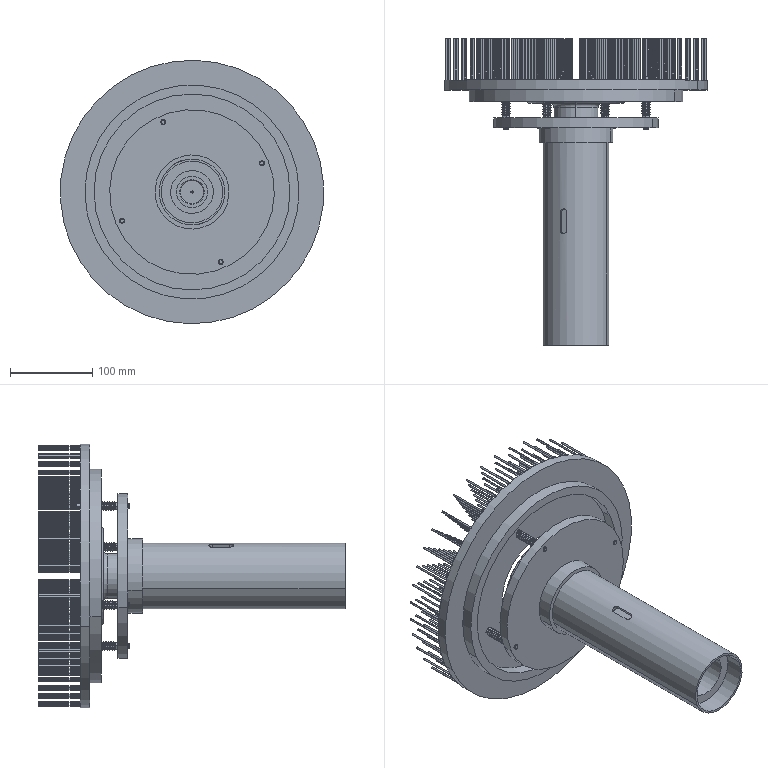Part | NX | features BREP 11 | 23 solids | 1564 faces | box 320 x 372 x 320 mm | volume 2233372 mm3 | cylinder 1010 | plane 502 | cone 32 | torus 12 | spline 8 | commonest cylinder face diameters 2 x800 2.5 x86 5 x30 6 x26 3.3 x12 9.238 x10